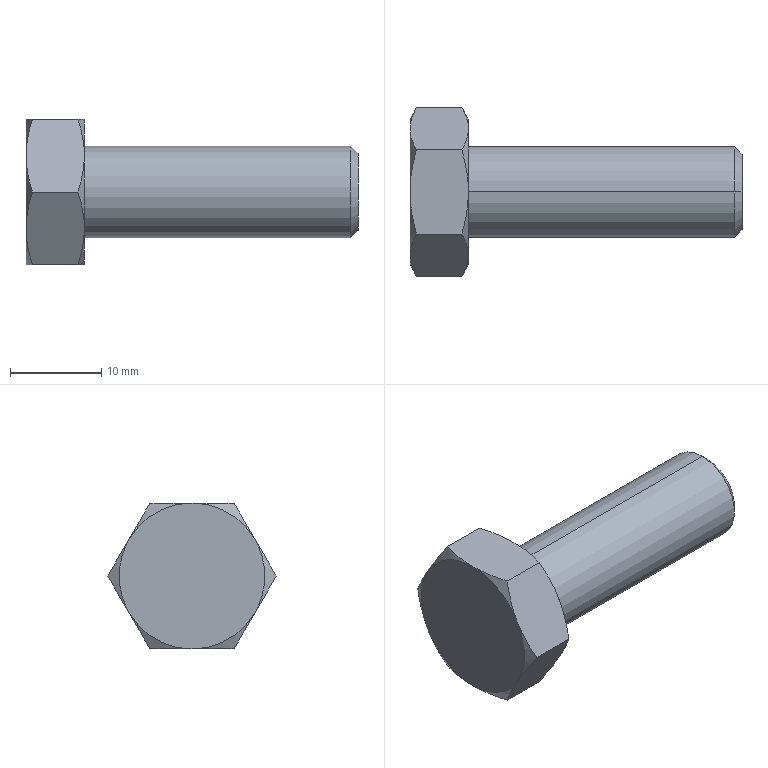Part | STEP file | Microwave Drying Flat Conveyor-screw_gb_t_6563_m10x30 | 1 solid | 25 faces | box 36.4 x 18.475 x 16 mm | volume 3756 mm3 | cone 14 | plane 9 | cylinder 2 | commonest cylinder face diameters 10 x2
STEP:
#1=CARTESIAN_POINT('',(30.,0.,4.188));
#2=VERTEX_POINT('',#1);
#3=CARTESIAN_POINT('',(30.,0.,-4.188));
#4=VERTEX_POINT('',#3);
#5=CARTESIAN_POINT('',(30.,0.,0.));
#6=DIRECTION('',(-1.,0.,0.));
#7=DIRECTION('',(0.,0.,1.));
#8=AXIS2_PLACEMENT_3D('',#5,#6,#7);
#9=CIRCLE('',#8,4.188);
#10=EDGE_CURVE('',#2,#4,#9,.T.);
#11=ORIENTED_EDGE('',*,*,#10,.T.);
#12=CARTESIAN_POINT('',(29.188,0.,-5.));
#13=VERTEX_POINT('',#12);
#14=CARTESIAN_POINT('',(29.188,0.,-5.));
#15=DIRECTION('',(-0.7071,0.,-0.7071));
#16=VECTOR('',#15,1000.);
#17=LINE('',#14,#16);
#18=EDGE_CURVE('',#4,#13,#17,.T.);
#19=ORIENTED_EDGE('',*,*,#18,.T.);
#20=CARTESIAN_POINT('',(29.188,0.,5.));
#21=VERTEX_POINT('',#20);
#22=CARTESIAN_POINT('',(29.188,0.,0.));
#23=DIRECTION('',(-1.,0.,0.));
#24=DIRECTION('',(0.,0.,1.));
#25=AXIS2_PLACEMENT_3D('',#22,#23,#24);
#26=CIRCLE('',#25,5.);
#27=EDGE_CURVE('',#21,#13,#26,.T.);
#28=ORIENTED_EDGE('',*,*,#27,.F.);
#29=CARTESIAN_POINT('',(29.188,0.,5.));
#30=DIRECTION('',(-0.7071,0.,0.7071));
#31=VECTOR('',#30,1000.);
#32=LINE('',#29,#31);
#33=EDGE_CURVE('',#2,#21,#32,.T.);
#34=ORIENTED_EDGE('',*,*,#33,.F.);
#35=EDGE_LOOP('',(#11,#19,#28,#34));
#36=FACE_OUTER_BOUND('',#35,.T.);
#37=CARTESIAN_POINT('',(29.188,0.,0.));
#38=DIRECTION('',(-1.,0.,0.));
#39=DIRECTION('',(0.,0.,1.));
#40=AXIS2_PLACEMENT_3D('',#37,#38,#39);
#41=CONICAL_SURFACE('',#40,5.,0.7854);
#42=ADVANCED_FACE('',(#36),#41,.T.);
#43=ORIENTED_EDGE('',*,*,#27,.T.);
#44=CARTESIAN_POINT('',(0.,0.,-5.));
#45=VERTEX_POINT('',#44);
#46=CARTESIAN_POINT('',(-0.1,0.,-5.));
#47=DIRECTION('',(-1.,0.,0.));
#48=VECTOR('',#47,1000.);
#49=LINE('',#46,#48);
#50=EDGE_CURVE('',#13,#45,#49,.T.);
#51=ORIENTED_EDGE('',*,*,#50,.T.);
#52=CARTESIAN_POINT('',(0.,0.,5.));
#53=VERTEX_POINT('',#52);
#54=CARTESIAN_POINT('',(0.,0.,0.));
#55=DIRECTION('',(1.,0.,0.));
#56=DIRECTION('',(0.,0.,1.));
#57=AXIS2_PLACEMENT_3D('',#54,#55,#56);
#58=CIRCLE('',#57,5.);
#59=EDGE_CURVE('',#45,#53,#58,.T.);
#60=ORIENTED_EDGE('',*,*,#59,.T.);
#61=CARTESIAN_POINT('',(-0.1,0.,5.));
#62=DIRECTION('',(-1.,0.,0.));
#63=VECTOR('',#62,1000.);
#64=LINE('',#61,#63);
#65=EDGE_CURVE('',#21,#53,#64,.T.);
#66=ORIENTED_EDGE('',*,*,#65,.F.);
#67=EDGE_LOOP('',(#43,#51,#60,#66));
#68=FACE_OUTER_BOUND('',#67,.T.);
#69=CARTESIAN_POINT('',(-0.1,0.,0.));
#70=DIRECTION('',(-1.,0.,0.));
#71=DIRECTION('',(0.,0.,1.));
#72=AXIS2_PLACEMENT_3D('',#69,#70,#71);
#73=CYLINDRICAL_SURFACE('',#72,5.);
#74=ADVANCED_FACE('',(#68),#73,.T.);
#75=ORIENTED_EDGE('',*,*,#50,.F.);
#76=CARTESIAN_POINT('',(29.188,0.,0.));
#77=DIRECTION('',(-1.,0.,0.));
#78=DIRECTION('',(0.,0.,1.));
#79=AXIS2_PLACEMENT_3D('',#76,#77,#78);
#80=CIRCLE('',#79,5.);
#81=EDGE_CURVE('',#13,#21,#80,.T.);
#82=ORIENTED_EDGE('',*,*,#81,.T.);
#83=ORIENTED_EDGE('',*,*,#65,.T.);
#84=CARTESIAN_POINT('',(0.,0.,0.));
#85=DIRECTION('',(1.,0.,0.));
#86=DIRECTION('',(0.,0.,1.));
#87=AXIS2_PLACEMENT_3D('',#84,#85,#86);
#88=CIRCLE('',#87,5.);
#89=EDGE_CURVE('',#53,#45,#88,.T.);
#90=ORIENTED_EDGE('',*,*,#89,.T.);
#91=EDGE_LOOP('',(#75,#82,#83,#90));
#92=FACE_OUTER_BOUND('',#91,.T.);
#93=CARTESIAN_POINT('',(-0.1,0.,0.));
#94=DIRECTION('',(-1.,0.,0.));
#95=DIRECTION('',(0.,0.,1.));
#96=AXIS2_PLACEMENT_3D('',#93,#94,#95);
#97=CYLINDRICAL_SURFACE('',#96,5.);
#98=ADVANCED_FACE('',(#92),#97,.T.);
#99=ORIENTED_EDGE('',*,*,#10,.F.);
#100=CARTESIAN_POINT('',(30.,0.,0.));
#101=DIRECTION('',(-1.,0.,0.));
#102=DIRECTION('',(0.,0.,1.));
#103=AXIS2_PLACEMENT_3D('',#100,#101,#102);
#104=CIRCLE('',#103,4.188);
#105=EDGE_CURVE('',#4,#2,#104,.T.);
#106=ORIENTED_EDGE('',*,*,#105,.F.);
#107=EDGE_LOOP('',(#99,#106));
#108=FACE_OUTER_BOUND('',#107,.T.);
#109=CARTESIAN_POINT('',(30.,0.,0.));
#110=DIRECTION('',(-1.,0.,0.));
#111=DIRECTION('',(0.,0.,1.));
#112=AXIS2_PLACEMENT_3D('',#109,#110,#111);
#113=PLANE('',#112);
#114=ADVANCED_FACE('',(#108),#113,.F.);
#115=ORIENTED_EDGE('',*,*,#18,.F.);
#116=ORIENTED_EDGE('',*,*,#105,.T.);
#117=ORIENTED_EDGE('',*,*,#33,.T.);
#118=ORIENTED_EDGE('',*,*,#81,.F.);
#119=EDGE_LOOP('',(#115,#116,#117,#118));
#120=FACE_OUTER_BOUND('',#119,.T.);
#121=CARTESIAN_POINT('',(29.188,0.,0.));
#122=DIRECTION('',(-1.,0.,0.));
#123=DIRECTION('',(0.,0.,1.));
#124=AXIS2_PLACEMENT_3D('',#121,#122,#123);
#125=CONICAL_SURFACE('',#124,5.,0.7854);
#126=ADVANCED_FACE('',(#120),#125,.T.);
#127=CARTESIAN_POINT('',(-0.7145,4.619,-8.));
#128=VERTEX_POINT('',#127);
#129=CARTESIAN_POINT('',(0.,0.,-8.));
#130=VERTEX_POINT('',#129);
#131=CARTESIAN_POINT('',(-0.7145,4.619,-8.));
#132=CARTESIAN_POINT('',(-0.4989,3.872,-8.));
#133=CARTESIAN_POINT('',(-0.3194,3.115,-8.));
#134=CARTESIAN_POINT('',(-0.1317,1.959,-8.));
#135=CARTESIAN_POINT('',(-0.08283,1.571,-8.));
#136=CARTESIAN_POINT('',(-0.01675,0.7849,-8.));
#137=CARTESIAN_POINT('',(0.,0.3912,-8.));
#138=CARTESIAN_POINT('',(0.,0.,-8.));
#139=B_SPLINE_CURVE_WITH_KNOTS('',3,(#131,#132,#133,#134,#135,#136,#137,#138),.UNSPECIFIED.,.F.,.F.,(4,2,2,4),(0.02228,0.02462,0.02579,0.02696),.UNSPECIFIED.);
#140=EDGE_CURVE('',#128,#130,#139,.T.);
#141=ORIENTED_EDGE('',*,*,#140,.F.);
#142=CARTESIAN_POINT('',(0.,6.928,-4.));
#143=VERTEX_POINT('',#142);
#144=CARTESIAN_POINT('',(0.,6.928,-4.));
#145=CARTESIAN_POINT('',(0.,6.732,-4.339));
#146=CARTESIAN_POINT('',(-0.01689,6.535,-4.68));
#147=CARTESIAN_POINT('',(-0.08225,6.146,-5.355));
#148=CARTESIAN_POINT('',(-0.1307,5.952,-5.69));
#149=CARTESIAN_POINT('',(-0.3174,5.376,-6.689));
#150=CARTESIAN_POINT('',(-0.497,4.996,-7.347));
#151=CARTESIAN_POINT('',(-0.7145,4.619,-8.));
#152=B_SPLINE_CURVE_WITH_KNOTS('',3,(#144,#145,#146,#147,#148,#149,#150,#151),.UNSPECIFIED.,.F.,.F.,(4,2,2,4),(0.004673,0.005837,0.007001,0.009329),.UNSPECIFIED.);
#153=EDGE_CURVE('',#143,#128,#152,.T.);
#154=ORIENTED_EDGE('',*,*,#153,.F.);
#155=CARTESIAN_POINT('',(0.,0.,0.));
#156=DIRECTION('',(-1.,0.,0.));
#157=DIRECTION('',(0.,0.,1.));
#158=AXIS2_PLACEMENT_3D('',#155,#156,#157);
#159=CIRCLE('',#158,8.);
#160=EDGE_CURVE('',#143,#130,#159,.T.);
#161=ORIENTED_EDGE('',*,*,#160,.T.);
#162=EDGE_LOOP('',(#141,#154,#161));
#163=FACE_OUTER_BOUND('',#162,.T.);
#164=CARTESIAN_POINT('',(0.,0.,0.));
#165=DIRECTION('',(-1.,0.,0.));
#166=DIRECTION('',(0.,0.,1.));
#167=AXIS2_PLACEMENT_3D('',#164,#165,#166);
#168=CONICAL_SURFACE('',#167,8.,1.047);
#169=ADVANCED_FACE('',(#163),#168,.T.);
#170=CARTESIAN_POINT('',(-0.7145,-4.619,-8.));
#171=VERTEX_POINT('',#170);
#172=CARTESIAN_POINT('',(0.,0.,-8.));
#173=CARTESIAN_POINT('',(0.,-0.7817,-8.));
#174=CARTESIAN_POINT('',(-0.06727,-1.557,-8.));
#175=CARTESIAN_POINT('',(-0.3157,-3.098,-8.));
#176=CARTESIAN_POINT('',(-0.4974,-3.866,-8.));
#177=CARTESIAN_POINT('',(-0.7145,-4.619,-8.));
#178=B_SPLINE_CURVE_WITH_KNOTS('',3,(#172,#173,#174,#175,#176,#177),.UNSPECIFIED.,.F.,.F.,(4,2,4),(0.02696,0.0293,0.03163),.UNSPECIFIED.);
#179=EDGE_CURVE('',#130,#171,#178,.T.);
#180=ORIENTED_EDGE('',*,*,#179,.F.);
#181=CARTESIAN_POINT('',(0.,-6.928,-4.));
#182=VERTEX_POINT('',#181);
#183=CARTESIAN_POINT('',(0.,0.,0.));
#184=DIRECTION('',(-1.,0.,0.));
#185=DIRECTION('',(0.,0.,1.));
#186=AXIS2_PLACEMENT_3D('',#183,#184,#185);
#187=CIRCLE('',#186,8.);
#188=EDGE_CURVE('',#130,#182,#187,.T.);
#189=ORIENTED_EDGE('',*,*,#188,.T.);
#190=CARTESIAN_POINT('',(-0.7145,-4.619,-8.));
#191=CARTESIAN_POINT('',(-0.4964,-4.997,-7.346));
#192=CARTESIAN_POINT('',(-0.3167,-5.377,-6.687));
#193=CARTESIAN_POINT('',(-0.0681,-6.146,-5.354));
#194=CARTESIAN_POINT('',(0.,-6.535,-4.681));
#195=CARTESIAN_POINT('',(0.,-6.928,-4.));
#196=B_SPLINE_CURVE_WITH_KNOTS('',3,(#190,#191,#192,#193,#194,#195),.UNSPECIFIED.,.F.,.F.,(4,2,4),(0.000000002,0.002337,0.004673),.UNSPECIFIED.);
#197=EDGE_CURVE('',#171,#182,#196,.T.);
#198=ORIENTED_EDGE('',*,*,#197,.F.);
#199=EDGE_LOOP('',(#180,#189,#198));
#200=FACE_OUTER_BOUND('',#199,.T.);
#201=CARTESIAN_POINT('',(0.,0.,0.));
#202=DIRECTION('',(-1.,0.,0.));
#203=DIRECTION('',(0.,0.,1.));
#204=AXIS2_PLACEMENT_3D('',#201,#202,#203);
#205=CONICAL_SURFACE('',#204,8.,1.047);
#206=ADVANCED_FACE('',(#200),#205,.T.);
#207=CARTESIAN_POINT('',(-0.7145,-9.238,0.));
#208=VERTEX_POINT('',#207);
#209=CARTESIAN_POINT('',(0.,-6.928,-4.));
#210=CARTESIAN_POINT('',(0.,-7.124,-3.661));
#211=CARTESIAN_POINT('',(-0.01689,-7.321,-3.32));
#212=CARTESIAN_POINT('',(-0.08225,-7.711,-2.645));
#213=CARTESIAN_POINT('',(-0.1307,-7.904,-2.31));
#214=CARTESIAN_POINT('',(-0.3174,-8.481,-1.311));
#215=CARTESIAN_POINT('',(-0.497,-8.861,-0.6527));
#216=CARTESIAN_POINT('',(-0.7145,-9.238,0.));
#217=B_SPLINE_CURVE_WITH_KNOTS('',3,(#209,#210,#211,#212,#213,#214,#215,#216),.UNSPECIFIED.,.F.,.F.,(4,2,2,4),(0.004673,0.005837,0.007001,0.009329),.UNSPECIFIED.);
#218=EDGE_CURVE('',#182,#208,#217,.T.);
#219=ORIENTED_EDGE('',*,*,#218,.F.);
#220=CARTESIAN_POINT('',(0.,-6.928,4.));
#221=VERTEX_POINT('',#220);
#222=CARTESIAN_POINT('',(0.,0.,0.));
#223=DIRECTION('',(-1.,0.,0.));
#224=DIRECTION('',(0.,0.,1.));
#225=AXIS2_PLACEMENT_3D('',#222,#223,#224);
#226=CIRCLE('',#225,8.);
#227=EDGE_CURVE('',#182,#221,#226,.T.);
#228=ORIENTED_EDGE('',*,*,#227,.T.);
#229=CARTESIAN_POINT('',(-0.7145,-9.238,0.));
#230=CARTESIAN_POINT('',(-0.4964,-8.86,0.6543));
#231=CARTESIAN_POINT('',(-0.3167,-8.479,1.313));
#232=CARTESIAN_POINT('',(-0.0681,-7.71,2.646));
#233=CARTESIAN_POINT('',(0.,-7.322,3.319));
#234=CARTESIAN_POINT('',(0.,-6.928,4.));
#235=B_SPLINE_CURVE_WITH_KNOTS('',3,(#229,#230,#231,#232,#233,#234),.UNSPECIFIED.,.F.,.F.,(4,2,4),(0.000000002,0.002337,0.004673),.UNSPECIFIED.);
#236=EDGE_CURVE('',#208,#221,#235,.T.);
#237=ORIENTED_EDGE('',*,*,#236,.F.);
#238=EDGE_LOOP('',(#219,#228,#237));
#239=FACE_OUTER_BOUND('',#238,.T.);
#240=CARTESIAN_POINT('',(0.,0.,0.));
#241=DIRECTION('',(-1.,0.,0.));
#242=DIRECTION('',(0.,0.,1.));
#243=AXIS2_PLACEMENT_3D('',#240,#241,#242);
#244=CONICAL_SURFACE('',#243,8.,1.047);
#245=ADVANCED_FACE('',(#239),#244,.T.);
#246=CARTESIAN_POINT('',(-0.7145,9.238,0.));
#247=VERTEX_POINT('',#246);
#248=CARTESIAN_POINT('',(-0.7145,9.238,0.));
#249=CARTESIAN_POINT('',(-0.4964,8.86,-0.6543));
#250=CARTESIAN_POINT('',(-0.3167,8.479,-1.313));
#251=CARTESIAN_POINT('',(-0.0681,7.71,-2.646));
#252=CARTESIAN_POINT('',(0.,7.322,-3.319));
#253=CARTESIAN_POINT('',(0.,6.928,-4.));
#254=B_SPLINE_CURVE_WITH_KNOTS('',3,(#248,#249,#250,#251,#252,#253),.UNSPECIFIED.,.F.,.F.,(4,2,4),(0.000000002,0.002337,0.004673),.UNSPECIFIED.);
#255=EDGE_CURVE('',#247,#143,#254,.T.);
#256=ORIENTED_EDGE('',*,*,#255,.F.);
#257=CARTESIAN_POINT('',(0.,6.928,4.));
#258=VERTEX_POINT('',#257);
#259=CARTESIAN_POINT('',(0.,6.928,4.));
#260=CARTESIAN_POINT('',(0.,7.124,3.661));
#261=CARTESIAN_POINT('',(-0.01689,7.321,3.32));
#262=CARTESIAN_POINT('',(-0.08225,7.711,2.645));
#263=CARTESIAN_POINT('',(-0.1307,7.904,2.31));
#264=CARTESIAN_POINT('',(-0.3174,8.481,1.311));
#265=CARTESIAN_POINT('',(-0.497,8.861,0.6527));
#266=CARTESIAN_POINT('',(-0.7145,9.238,0.));
#267=B_SPLINE_CURVE_WITH_KNOTS('',3,(#259,#260,#261,#262,#263,#264,#265,#266),.UNSPECIFIED.,.F.,.F.,(4,2,2,4),(0.004673,0.005837,0.007001,0.009329),.UNSPECIFIED.);
#268=EDGE_CURVE('',#258,#247,#267,.T.);
#269=ORIENTED_EDGE('',*,*,#268,.F.);
#270=CARTESIAN_POINT('',(0.,0.,0.));
#271=DIRECTION('',(-1.,0.,0.));
#272=DIRECTION('',(0.,0.,1.));
#273=AXIS2_PLACEMENT_3D('',#270,#271,#272);
#274=CIRCLE('',#273,8.);
#275=EDGE_CURVE('',#258,#143,#274,.T.);
#276=ORIENTED_EDGE('',*,*,#275,.T.);
#277=EDGE_LOOP('',(#256,#269,#276));
#278=FACE_OUTER_BOUND('',#277,.T.);
#279=CARTESIAN_POINT('',(0.,0.,0.));
#280=DIRECTION('',(-1.,0.,0.));
#281=DIRECTION('',(0.,0.,1.));
#282=AXIS2_PLACEMENT_3D('',#279,#280,#281);
#283=CONICAL_SURFACE('',#282,8.,1.047);
#284=ADVANCED_FACE('',(#278),#283,.T.);
#285=CARTESIAN_POINT('',(-0.7145,-4.619,8.));
#286=VERTEX_POINT('',#285);
#287=CARTESIAN_POINT('',(0.,-6.928,4.));
#288=CARTESIAN_POINT('',(0.,-6.732,4.339));
#289=CARTESIAN_POINT('',(-0.01689,-6.535,4.68));
#290=CARTESIAN_POINT('',(-0.08225,-6.146,5.355));
#291=CARTESIAN_POINT('',(-0.1307,-5.952,5.69));
#292=CARTESIAN_POINT('',(-0.3174,-5.376,6.689));
#293=CARTESIAN_POINT('',(-0.497,-4.996,7.347));
#294=CARTESIAN_POINT('',(-0.7145,-4.619,8.));
#295=B_SPLINE_CURVE_WITH_KNOTS('',3,(#287,#288,#289,#290,#291,#292,#293,#294),.UNSPECIFIED.,.F.,.F.,(4,2,2,4),(0.004673,0.005837,0.007001,0.009329),.UNSPECIFIED.);
#296=EDGE_CURVE('',#221,#286,#295,.T.);
#297=ORIENTED_EDGE('',*,*,#296,.F.);
#298=CARTESIAN_POINT('',(0.,0.,8.));
#299=VERTEX_POINT('',#298);
#300=CARTESIAN_POINT('',(0.,0.,0.));
#301=DIRECTION('',(-1.,0.,0.));
#302=DIRECTION('',(0.,0.,1.));
#303=AXIS2_PLACEMENT_3D('',#300,#301,#302);
#304=CIRCLE('',#303,8.);
#305=EDGE_CURVE('',#221,#299,#304,.T.);
#306=ORIENTED_EDGE('',*,*,#305,.T.);
#307=CARTESIAN_POINT('',(-0.7145,-4.619,8.));
#308=CARTESIAN_POINT('',(-0.4974,-3.866,8.));
#309=CARTESIAN_POINT('',(-0.3157,-3.098,8.));
#310=CARTESIAN_POINT('',(-0.06727,-1.557,8.));
#311=CARTESIAN_POINT('',(0.,-0.7817,8.));
#312=CARTESIAN_POINT('',(0.,0.,8.));
#313=B_SPLINE_CURVE_WITH_KNOTS('',3,(#307,#308,#309,#310,#311,#312),.UNSPECIFIED.,.F.,.F.,(4,2,4),(0.008627,0.01097,0.0133),.UNSPECIFIED.);
#314=EDGE_CURVE('',#286,#299,#313,.T.);
#315=ORIENTED_EDGE('',*,*,#314,.F.);
#316=EDGE_LOOP('',(#297,#306,#315));
#317=FACE_OUTER_BOUND('',#316,.T.);
#318=CARTESIAN_POINT('',(0.,0.,0.));
#319=DIRECTION('',(-1.,0.,0.));
#320=DIRECTION('',(0.,0.,1.));
#321=AXIS2_PLACEMENT_3D('',#318,#319,#320);
#322=CONICAL_SURFACE('',#321,8.,1.047);
#323=ADVANCED_FACE('',(#317),#322,.T.);
#324=CARTESIAN_POINT('',(-0.7145,4.619,8.));
#325=VERTEX_POINT('',#324);
#326=CARTESIAN_POINT('',(-0.7145,4.619,8.));
#327=CARTESIAN_POINT('',(-0.4964,4.997,7.346));
#328=CARTESIAN_POINT('',(-0.3167,5.377,6.687));
#329=CARTESIAN_POINT('',(-0.0681,6.146,5.354));
#330=CARTESIAN_POINT('',(0.,6.535,4.681));
#331=CARTESIAN_POINT('',(0.,6.928,4.));
#332=B_SPLINE_CURVE_WITH_KNOTS('',3,(#326,#327,#328,#329,#330,#331),.UNSPECIFIED.,.F.,.F.,(4,2,4),(0.000000002,0.002337,0.004673),.UNSPECIFIED.);
#333=EDGE_CURVE('',#325,#258,#332,.T.);
#334=ORIENTED_EDGE('',*,*,#333,.F.);
#335=CARTESIAN_POINT('',(0.,0.,8.));
#336=CARTESIAN_POINT('',(0.,0.3912,8.));
#337=CARTESIAN_POINT('',(-0.01675,0.7849,8.));
#338=CARTESIAN_POINT('',(-0.08283,1.571,8.));
#339=CARTESIAN_POINT('',(-0.1317,1.959,8.));
#340=CARTESIAN_POINT('',(-0.3194,3.115,8.));
#341=CARTESIAN_POINT('',(-0.4989,3.872,8.));
#342=CARTESIAN_POINT('',(-0.7145,4.619,8.));
#343=B_SPLINE_CURVE_WITH_KNOTS('',3,(#335,#336,#337,#338,#339,#340,#341,#342),.UNSPECIFIED.,.F.,.F.,(4,2,2,4),(0.0133,0.01447,0.01564,0.01798),.UNSPECIFIED.);
#344=EDGE_CURVE('',#299,#325,#343,.T.);
#345=ORIENTED_EDGE('',*,*,#344,.F.);
#346=CARTESIAN_POINT('',(0.,0.,0.));
#347=DIRECTION('',(-1.,0.,0.));
#348=DIRECTION('',(0.,0.,1.));
#349=AXIS2_PLACEMENT_3D('',#346,#347,#348);
#350=CIRCLE('',#349,8.);
#351=EDGE_CURVE('',#299,#258,#350,.T.);
#352=ORIENTED_EDGE('',*,*,#351,.T.);
#353=EDGE_LOOP('',(#334,#345,#352));
#354=FACE_OUTER_BOUND('',#353,.T.);
#355=CARTESIAN_POINT('',(0.,0.,0.));
#356=DIRECTION('',(-1.,0.,0.));
#357=DIRECTION('',(0.,0.,1.));
#358=AXIS2_PLACEMENT_3D('',#355,#356,#357);
#359=CONICAL_SURFACE('',#358,8.,1.047);
#360=ADVANCED_FACE('',(#354),#359,.T.);
#361=ORIENTED_EDGE('',*,*,#89,.F.);
#362=ORIENTED_EDGE('',*,*,#59,.F.);
#363=EDGE_LOOP('',(#361,#362));
#364=FACE_BOUND('',#363,.T.);
#365=ORIENTED_EDGE('',*,*,#351,.F.);
#366=ORIENTED_EDGE('',*,*,#305,.F.);
#367=ORIENTED_EDGE('',*,*,#227,.F.);
#368=ORIENTED_EDGE('',*,*,#188,.F.);
#369=ORIENTED_EDGE('',*,*,#160,.F.);
#370=ORIENTED_EDGE('',*,*,#275,.F.);
#371=EDGE_LOOP('',(#365,#366,#367,#368,#369,#370));
#372=FACE_OUTER_BOUND('',#371,.T.);
#373=CARTESIAN_POINT('',(0.,0.,0.));
#374=DIRECTION('',(-1.,0.,0.));
#375=DIRECTION('',(0.,0.,1.));
#376=AXIS2_PLACEMENT_3D('',#373,#374,#375);
#377=PLANE('',#376);
#378=ADVANCED_FACE('',(#364,#372),#377,.F.);
#379=CARTESIAN_POINT('',(-5.685,-9.238,0.));
#380=VERTEX_POINT('',#379);
#381=CARTESIAN_POINT('',(0.2,-9.238,0.));
#382=DIRECTION('',(-1.,0.,0.));
#383=VECTOR('',#382,1000.);
#384=LINE('',#381,#383);
#385=EDGE_CURVE('',#208,#380,#384,.T.);
#386=ORIENTED_EDGE('',*,*,#385,.F.);
#387=ORIENTED_EDGE('',*,*,#236,.T.);
#388=ORIENTED_EDGE('',*,*,#296,.T.);
#389=CARTESIAN_POINT('',(-5.685,-4.619,8.));
#390=VERTEX_POINT('',#389);
#391=CARTESIAN_POINT('',(0.2,-4.619,8.));
#392=DIRECTION('',(-1.,0.,0.));
#393=VECTOR('',#392,1000.);
#394=LINE('',#391,#393);
#395=EDGE_CURVE('',#286,#390,#394,.T.);
#396=ORIENTED_EDGE('',*,*,#395,.T.);
#397=CARTESIAN_POINT('',(-6.4,-6.928,4.));
#398=VERTEX_POINT('',#397);
#399=CARTESIAN_POINT('',(-6.4,-6.928,4.));
#400=CARTESIAN_POINT('',(-6.4,-6.732,4.339));
#401=CARTESIAN_POINT('',(-6.383,-6.535,4.68));
#402=CARTESIAN_POINT('',(-6.318,-6.146,5.355));
#403=CARTESIAN_POINT('',(-6.269,-5.952,5.69));
#404=CARTESIAN_POINT('',(-6.083,-5.376,6.689));
#405=CARTESIAN_POINT('',(-5.903,-4.996,7.347));
#406=CARTESIAN_POINT('',(-5.685,-4.619,8.));
#407=B_SPLINE_CURVE_WITH_KNOTS('',3,(#399,#400,#401,#402,#403,#404,#405,#406),.UNSPECIFIED.,.F.,.F.,(4,2,2,4),(0.004673,0.005837,0.007001,0.009329),.UNSPECIFIED.);
#408=EDGE_CURVE('',#398,#390,#407,.T.);
#409=ORIENTED_EDGE('',*,*,#408,.F.);
#410=CARTESIAN_POINT('',(-5.685,-9.238,0.));
#411=CARTESIAN_POINT('',(-5.904,-8.86,0.6543));
#412=CARTESIAN_POINT('',(-6.083,-8.479,1.313));
#413=CARTESIAN_POINT('',(-6.332,-7.71,2.646));
#414=CARTESIAN_POINT('',(-6.4,-7.322,3.319));
#415=CARTESIAN_POINT('',(-6.4,-6.928,4.));
#416=B_SPLINE_CURVE_WITH_KNOTS('',3,(#410,#411,#412,#413,#414,#415),.UNSPECIFIED.,.F.,.F.,(4,2,4),(0.000000002,0.002337,0.004673),.UNSPECIFIED.);
#417=EDGE_CURVE('',#380,#398,#416,.T.);
#418=ORIENTED_EDGE('',*,*,#417,.F.);
#419=EDGE_LOOP('',(#386,#387,#388,#396,#409,#418));
#420=FACE_OUTER_BOUND('',#419,.T.);
#421=CARTESIAN_POINT('',(0.2,-4.619,8.));
#422=DIRECTION('',(0.,0.866,-0.5));
#423=DIRECTION('',(0.,0.5,0.866));
#424=AXIS2_PLACEMENT_3D('',#421,#422,#423);
#425=PLANE('',#424);
#426=ADVANCED_FACE('',(#420),#425,.F.);
#427=CARTESIAN_POINT('',(-5.685,-4.619,-8.));
#428=VERTEX_POINT('',#427);
#429=CARTESIAN_POINT('',(0.2,-4.619,-8.));
#430=DIRECTION('',(-1.,0.,0.));
#431=VECTOR('',#430,1000.);
#432=LINE('',#429,#431);
#433=EDGE_CURVE('',#171,#428,#432,.T.);
#434=ORIENTED_EDGE('',*,*,#433,.F.);
#435=ORIENTED_EDGE('',*,*,#197,.T.);
#436=ORIENTED_EDGE('',*,*,#218,.T.);
#437=ORIENTED_EDGE('',*,*,#385,.T.);
#438=CARTESIAN_POINT('',(-6.4,-6.928,-4.));
#439=VERTEX_POINT('',#438);
#440=CARTESIAN_POINT('',(-6.4,-6.928,-4.));
#441=CARTESIAN_POINT('',(-6.4,-7.124,-3.661));
#442=CARTESIAN_POINT('',(-6.383,-7.321,-3.32));
#443=CARTESIAN_POINT('',(-6.318,-7.711,-2.645));
#444=CARTESIAN_POINT('',(-6.269,-7.904,-2.31));
#445=CARTESIAN_POINT('',(-6.083,-8.481,-1.311));
#446=CARTESIAN_POINT('',(-5.903,-8.861,-0.6527));
#447=CARTESIAN_POINT('',(-5.685,-9.238,0.));
#448=B_SPLINE_CURVE_WITH_KNOTS('',3,(#440,#441,#442,#443,#444,#445,#446,#447),.UNSPECIFIED.,.F.,.F.,(4,2,2,4),(0.004673,0.005837,0.007001,0.009329),.UNSPECIFIED.);
#449=EDGE_CURVE('',#439,#380,#448,.T.);
#450=ORIENTED_EDGE('',*,*,#449,.F.);
#451=CARTESIAN_POINT('',(-5.685,-4.619,-8.));
#452=CARTESIAN_POINT('',(-5.904,-4.997,-7.346));
#453=CARTESIAN_POINT('',(-6.083,-5.377,-6.687));
#454=CARTESIAN_POINT('',(-6.332,-6.146,-5.354));
#455=CARTESIAN_POINT('',(-6.4,-6.535,-4.681));
#456=CARTESIAN_POINT('',(-6.4,-6.928,-4.));
#457=B_SPLINE_CURVE_WITH_KNOTS('',3,(#451,#452,#453,#454,#455,#456),.UNSPECIFIED.,.F.,.F.,(4,2,4),(0.000000002,0.002337,0.004673),.UNSPECIFIED.);
#458=EDGE_CURVE('',#428,#439,#457,.T.);
#459=ORIENTED_EDGE('',*,*,#458,.F.);
#460=EDGE_LOOP('',(#434,#435,#436,#437,#450,#459));
#461=FACE_OUTER_BOUND('',#460,.T.);
#462=CARTESIAN_POINT('',(0.2,-9.238,0.));
#463=DIRECTION('',(0.,0.866,0.5));
#464=DIRECTION('',(0.,-0.5,0.866));
#465=AXIS2_PLACEMENT_3D('',#462,#463,#464);
#466=PLANE('',#465);
#467=ADVANCED_FACE('',(#461),#466,.F.);
#468=CARTESIAN_POINT('',(-5.685,4.619,-8.));
#469=VERTEX_POINT('',#468);
#470=CARTESIAN_POINT('',(0.2,4.619,-8.));
#471=DIRECTION('',(-1.,0.,0.));
#472=VECTOR('',#471,1000.);
#473=LINE('',#470,#472);
#474=EDGE_CURVE('',#128,#469,#473,.T.);
#475=ORIENTED_EDGE('',*,*,#474,.F.);
#476=ORIENTED_EDGE('',*,*,#140,.T.);
#477=ORIENTED_EDGE('',*,*,#179,.T.);
#478=ORIENTED_EDGE('',*,*,#433,.T.);
#479=CARTESIAN_POINT('',(-6.4,0.,-8.));
#480=VERTEX_POINT('',#479);
#481=CARTESIAN_POINT('',(-6.4,0.,-8.));
#482=CARTESIAN_POINT('',(-6.4,-0.7817,-8.));
#483=CARTESIAN_POINT('',(-6.333,-1.557,-8.));
#484=CARTESIAN_POINT('',(-6.084,-3.098,-8.));
#485=CARTESIAN_POINT('',(-5.903,-3.866,-8.));
#486=CARTESIAN_POINT('',(-5.685,-4.619,-8.));
#487=B_SPLINE_CURVE_WITH_KNOTS('',3,(#481,#482,#483,#484,#485,#486),.UNSPECIFIED.,.F.,.F.,(4,2,4),(0.02696,0.0293,0.03163),.UNSPECIFIED.);
#488=EDGE_CURVE('',#480,#428,#487,.T.);
#489=ORIENTED_EDGE('',*,*,#488,.F.);
#490=CARTESIAN_POINT('',(-5.685,4.619,-8.));
#491=CARTESIAN_POINT('',(-5.901,3.872,-8.));
#492=CARTESIAN_POINT('',(-6.081,3.115,-8.));
#493=CARTESIAN_POINT('',(-6.268,1.959,-8.));
#494=CARTESIAN_POINT('',(-6.317,1.571,-8.));
#495=CARTESIAN_POINT('',(-6.383,0.7849,-8.));
#496=CARTESIAN_POINT('',(-6.4,0.3912,-8.));
#497=CARTESIAN_POINT('',(-6.4,0.,-8.));
#498=B_SPLINE_CURVE_WITH_KNOTS('',3,(#490,#491,#492,#493,#494,#495,#496,#497),.UNSPECIFIED.,.F.,.F.,(4,2,2,4),(0.02228,0.02462,0.02579,0.02696),.UNSPECIFIED.);
#499=EDGE_CURVE('',#469,#480,#498,.T.);
#500=ORIENTED_EDGE('',*,*,#499,.F.);
#501=EDGE_LOOP('',(#475,#476,#477,#478,#489,#500));
#502=FACE_OUTER_BOUND('',#501,.T.);
#503=CARTESIAN_POINT('',(0.2,-4.619,-8.));
#504=DIRECTION('',(0.,0.,1.));
#505=DIRECTION('',(0.,-1.,0.));
#506=AXIS2_PLACEMENT_3D('',#503,#504,#505);
#507=PLANE('',#506);
#508=ADVANCED_FACE('',(#502),#507,.F.);
#509=CARTESIAN_POINT('',(-5.685,9.238,0.));
#510=VERTEX_POINT('',#509);
#511=CARTESIAN_POINT('',(0.2,9.238,0.));
#512=DIRECTION('',(-1.,0.,0.));
#513=VECTOR('',#512,1000.);
#514=LINE('',#511,#513);
#515=EDGE_CURVE('',#247,#510,#514,.T.);
#516=ORIENTED_EDGE('',*,*,#515,.F.);
#517=ORIENTED_EDGE('',*,*,#255,.T.);
#518=ORIENTED_EDGE('',*,*,#153,.T.);
#519=ORIENTED_EDGE('',*,*,#474,.T.);
#520=CARTESIAN_POINT('',(-6.4,6.928,-4.));
#521=VERTEX_POINT('',#520);
#522=CARTESIAN_POINT('',(-6.4,6.928,-4.));
#523=CARTESIAN_POINT('',(-6.4,6.732,-4.339));
#524=CARTESIAN_POINT('',(-6.383,6.535,-4.68));
#525=CARTESIAN_POINT('',(-6.318,6.146,-5.355));
#526=CARTESIAN_POINT('',(-6.269,5.952,-5.69));
#527=CARTESIAN_POINT('',(-6.083,5.376,-6.689));
#528=CARTESIAN_POINT('',(-5.903,4.996,-7.347));
#529=CARTESIAN_POINT('',(-5.685,4.619,-8.));
#530=B_SPLINE_CURVE_WITH_KNOTS('',3,(#522,#523,#524,#525,#526,#527,#528,#529),.UNSPECIFIED.,.F.,.F.,(4,2,2,4),(0.004673,0.005837,0.007001,0.009329),.UNSPECIFIED.);
#531=EDGE_CURVE('',#521,#469,#530,.T.);
#532=ORIENTED_EDGE('',*,*,#531,.F.);
#533=CARTESIAN_POINT('',(-5.685,9.238,0.));
#534=CARTESIAN_POINT('',(-5.904,8.86,-0.6543));
#535=CARTESIAN_POINT('',(-6.083,8.479,-1.313));
#536=CARTESIAN_POINT('',(-6.332,7.71,-2.646));
#537=CARTESIAN_POINT('',(-6.4,7.322,-3.319));
#538=CARTESIAN_POINT('',(-6.4,6.928,-4.));
#539=B_SPLINE_CURVE_WITH_KNOTS('',3,(#533,#534,#535,#536,#537,#538),.UNSPECIFIED.,.F.,.F.,(4,2,4),(0.000000002,0.002337,0.004673),.UNSPECIFIED.);
#540=EDGE_CURVE('',#510,#521,#539,.T.);
#541=ORIENTED_EDGE('',*,*,#540,.F.);
#542=EDGE_LOOP('',(#516,#517,#518,#519,#532,#541));
#543=FACE_OUTER_BOUND('',#542,.T.);
#544=CARTESIAN_POINT('',(0.2,4.619,-8.));
#545=DIRECTION('',(0.,-0.866,0.5));
#546=DIRECTION('',(0.,-0.5,-0.866));
#547=AXIS2_PLACEMENT_3D('',#544,#545,#546);
#548=PLANE('',#547);
#549=ADVANCED_FACE('',(#543),#548,.F.);
#550=CARTESIAN_POINT('',(-5.685,4.619,8.));
#551=VERTEX_POINT('',#550);
#552=CARTESIAN_POINT('',(0.2,4.619,8.));
#553=DIRECTION('',(-1.,0.,0.));
#554=VECTOR('',#553,1000.);
#555=LINE('',#552,#554);
#556=EDGE_CURVE('',#325,#551,#555,.T.);
#557=ORIENTED_EDGE('',*,*,#556,.F.);
#558=ORIENTED_EDGE('',*,*,#333,.T.);
#559=ORIENTED_EDGE('',*,*,#268,.T.);
#560=ORIENTED_EDGE('',*,*,#515,.T.);
#561=CARTESIAN_POINT('',(-6.4,6.928,4.));
#562=VERTEX_POINT('',#561);
#563=CARTESIAN_POINT('',(-6.4,6.928,4.));
#564=CARTESIAN_POINT('',(-6.4,7.124,3.661));
#565=CARTESIAN_POINT('',(-6.383,7.321,3.32));
#566=CARTESIAN_POINT('',(-6.318,7.711,2.645));
#567=CARTESIAN_POINT('',(-6.269,7.904,2.31));
#568=CARTESIAN_POINT('',(-6.083,8.481,1.311));
#569=CARTESIAN_POINT('',(-5.903,8.861,0.6527));
#570=CARTESIAN_POINT('',(-5.685,9.238,0.));
#571=B_SPLINE_CURVE_WITH_KNOTS('',3,(#563,#564,#565,#566,#567,#568,#569,#570),.UNSPECIFIED.,.F.,.F.,(4,2,2,4),(0.004673,0.005837,0.007001,0.009329),.UNSPECIFIED.);
#572=EDGE_CURVE('',#562,#510,#571,.T.);
#573=ORIENTED_EDGE('',*,*,#572,.F.);
#574=CARTESIAN_POINT('',(-5.685,4.619,8.));
#575=CARTESIAN_POINT('',(-5.904,4.997,7.346));
#576=CARTESIAN_POINT('',(-6.083,5.377,6.687));
#577=CARTESIAN_POINT('',(-6.332,6.146,5.354));
#578=CARTESIAN_POINT('',(-6.4,6.535,4.681));
#579=CARTESIAN_POINT('',(-6.4,6.928,4.));
#580=B_SPLINE_CURVE_WITH_KNOTS('',3,(#574,#575,#576,#577,#578,#579),.UNSPECIFIED.,.F.,.F.,(4,2,4),(0.000000002,0.002337,0.004673),.UNSPECIFIED.);
#581=EDGE_CURVE('',#551,#562,#580,.T.);
#582=ORIENTED_EDGE('',*,*,#581,.F.);
#583=EDGE_LOOP('',(#557,#558,#559,#560,#573,#582));
#584=FACE_OUTER_BOUND('',#583,.T.);
#585=CARTESIAN_POINT('',(0.2,9.238,0.));
#586=DIRECTION('',(0.,-0.866,-0.5));
#587=DIRECTION('',(0.,0.5,-0.866));
#588=AXIS2_PLACEMENT_3D('',#585,#586,#587);
#589=PLANE('',#588);
#590=ADVANCED_FACE('',(#584),#589,.F.);
#591=ORIENTED_EDGE('',*,*,#395,.F.);
#592=ORIENTED_EDGE('',*,*,#314,.T.);
#593=ORIENTED_EDGE('',*,*,#344,.T.);
#594=ORIENTED_EDGE('',*,*,#556,.T.);
#595=CARTESIAN_POINT('',(-6.4,0.,8.));
#596=VERTEX_POINT('',#595);
#597=CARTESIAN_POINT('',(-6.4,0.,8.));
#598=CARTESIAN_POINT('',(-6.4,0.3912,8.));
#599=CARTESIAN_POINT('',(-6.383,0.7849,8.));
#600=CARTESIAN_POINT('',(-6.317,1.571,8.));
#601=CARTESIAN_POINT('',(-6.268,1.959,8.));
#602=CARTESIAN_POINT('',(-6.081,3.115,8.));
#603=CARTESIAN_POINT('',(-5.901,3.872,8.));
#604=CARTESIAN_POINT('',(-5.685,4.619,8.));
#605=B_SPLINE_CURVE_WITH_KNOTS('',3,(#597,#598,#599,#600,#601,#602,#603,#604),.UNSPECIFIED.,.F.,.F.,(4,2,2,4),(0.0133,0.01447,0.01564,0.01798),.UNSPECIFIED.);
#606=EDGE_CURVE('',#596,#551,#605,.T.);
#607=ORIENTED_EDGE('',*,*,#606,.F.);
#608=CARTESIAN_POINT('',(-5.685,-4.619,8.));
#609=CARTESIAN_POINT('',(-5.903,-3.866,8.));
#610=CARTESIAN_POINT('',(-6.084,-3.098,8.));
#611=CARTESIAN_POINT('',(-6.333,-1.557,8.));
#612=CARTESIAN_POINT('',(-6.4,-0.7817,8.));
#613=CARTESIAN_POINT('',(-6.4,0.,8.));
#614=B_SPLINE_CURVE_WITH_KNOTS('',3,(#608,#609,#610,#611,#612,#613),.UNSPECIFIED.,.F.,.F.,(4,2,4),(0.008627,0.01097,0.0133),.UNSPECIFIED.);
#615=EDGE_CURVE('',#390,#596,#614,.T.);
#616=ORIENTED_EDGE('',*,*,#615,.F.);
#617=EDGE_LOOP('',(#591,#592,#593,#594,#607,#616));
#618=FACE_OUTER_BOUND('',#617,.T.);
#619=CARTESIAN_POINT('',(0.2,4.619,8.));
#620=DIRECTION('',(0.,0.,-1.));
#621=DIRECTION('',(0.,1.,0.));
#622=AXIS2_PLACEMENT_3D('',#619,#620,#621);
#623=PLANE('',#622);
#624=ADVANCED_FACE('',(#618),#623,.F.);
#625=CARTESIAN_POINT('',(-6.4,0.,0.));
#626=DIRECTION('',(-1.,0.,0.));
#627=DIRECTION('',(0.,0.,1.));
#628=AXIS2_PLACEMENT_3D('',#625,#626,#627);
#629=CIRCLE('',#628,8.);
#630=EDGE_CURVE('',#398,#596,#629,.T.);
#631=ORIENTED_EDGE('',*,*,#630,.F.);
#632=ORIENTED_EDGE('',*,*,#408,.T.);
#633=ORIENTED_EDGE('',*,*,#615,.T.);
#634=EDGE_LOOP('',(#631,#632,#633));
#635=FACE_OUTER_BOUND('',#634,.T.);
#636=CARTESIAN_POINT('',(-6.4,0.,0.));
#637=DIRECTION('',(1.,0.,0.));
#638=DIRECTION('',(0.,0.,-1.));
#639=AXIS2_PLACEMENT_3D('',#636,#637,#638);
#640=CONICAL_SURFACE('',#639,8.,1.047);
#641=ADVANCED_FACE('',(#635),#640,.T.);
#642=CARTESIAN_POINT('',(-6.4,0.,0.));
#643=DIRECTION('',(-1.,0.,0.));
#644=DIRECTION('',(0.,0.,1.));
#645=AXIS2_PLACEMENT_3D('',#642,#643,#644);
#646=CIRCLE('',#645,8.);
#647=EDGE_CURVE('',#439,#398,#646,.T.);
#648=ORIENTED_EDGE('',*,*,#647,.F.);
#649=ORIENTED_EDGE('',*,*,#449,.T.);
#650=ORIENTED_EDGE('',*,*,#417,.T.);
#651=EDGE_LOOP('',(#648,#649,#650));
#652=FACE_OUTER_BOUND('',#651,.T.);
#653=CARTESIAN_POINT('',(-6.4,0.,0.));
#654=DIRECTION('',(1.,0.,0.));
#655=DIRECTION('',(0.,0.,-1.));
#656=AXIS2_PLACEMENT_3D('',#653,#654,#655);
#657=CONICAL_SURFACE('',#656,8.,1.047);
#658=ADVANCED_FACE('',(#652),#657,.T.);
#659=CARTESIAN_POINT('',(-6.4,0.,0.));
#660=DIRECTION('',(-1.,0.,0.));
#661=DIRECTION('',(0.,0.,1.));
#662=AXIS2_PLACEMENT_3D('',#659,#660,#661);
#663=CIRCLE('',#662,8.);
#664=EDGE_CURVE('',#480,#439,#663,.T.);
#665=ORIENTED_EDGE('',*,*,#664,.F.);
#666=ORIENTED_EDGE('',*,*,#488,.T.);
#667=ORIENTED_EDGE('',*,*,#458,.T.);
#668=EDGE_LOOP('',(#665,#666,#667));
#669=FACE_OUTER_BOUND('',#668,.T.);
#670=CARTESIAN_POINT('',(-6.4,0.,0.));
#671=DIRECTION('',(1.,0.,0.));
#672=DIRECTION('',(0.,0.,-1.));
#673=AXIS2_PLACEMENT_3D('',#670,#671,#672);
#674=CONICAL_SURFACE('',#673,8.,1.047);
#675=ADVANCED_FACE('',(#669),#674,.T.);
#676=ORIENTED_EDGE('',*,*,#531,.T.);
#677=ORIENTED_EDGE('',*,*,#499,.T.);
#678=CARTESIAN_POINT('',(-6.4,0.,0.));
#679=DIRECTION('',(-1.,0.,0.));
#680=DIRECTION('',(0.,0.,1.));
#681=AXIS2_PLACEMENT_3D('',#678,#679,#680);
#682=CIRCLE('',#681,8.);
#683=EDGE_CURVE('',#521,#480,#682,.T.);
#684=ORIENTED_EDGE('',*,*,#683,.F.);
#685=EDGE_LOOP('',(#676,#677,#684));
#686=FACE_OUTER_BOUND('',#685,.T.);
#687=CARTESIAN_POINT('',(-6.4,0.,0.));
#688=DIRECTION('',(1.,0.,0.));
#689=DIRECTION('',(0.,0.,-1.));
#690=AXIS2_PLACEMENT_3D('',#687,#688,#689);
#691=CONICAL_SURFACE('',#690,8.,1.047);
#692=ADVANCED_FACE('',(#686),#691,.T.);
#693=ORIENTED_EDGE('',*,*,#572,.T.);
#694=ORIENTED_EDGE('',*,*,#540,.T.);
#695=CARTESIAN_POINT('',(-6.4,0.,0.));
#696=DIRECTION('',(-1.,0.,0.));
#697=DIRECTION('',(0.,0.,1.));
#698=AXIS2_PLACEMENT_3D('',#695,#696,#697);
#699=CIRCLE('',#698,8.);
#700=EDGE_CURVE('',#562,#521,#699,.T.);
#701=ORIENTED_EDGE('',*,*,#700,.F.);
#702=EDGE_LOOP('',(#693,#694,#701));
#703=FACE_OUTER_BOUND('',#702,.T.);
#704=CARTESIAN_POINT('',(-6.4,0.,0.));
#705=DIRECTION('',(1.,0.,0.));
#706=DIRECTION('',(0.,0.,-1.));
#707=AXIS2_PLACEMENT_3D('',#704,#705,#706);
#708=CONICAL_SURFACE('',#707,8.,1.047);
#709=ADVANCED_FACE('',(#703),#708,.T.);
#710=CARTESIAN_POINT('',(-6.4,0.,0.));
#711=DIRECTION('',(-1.,0.,0.));
#712=DIRECTION('',(0.,0.,1.));
#713=AXIS2_PLACEMENT_3D('',#710,#711,#712);
#714=CIRCLE('',#713,8.);
#715=EDGE_CURVE('',#596,#562,#714,.T.);
#716=ORIENTED_EDGE('',*,*,#715,.T.);
#717=ORIENTED_EDGE('',*,*,#700,.T.);
#718=ORIENTED_EDGE('',*,*,#683,.T.);
#719=ORIENTED_EDGE('',*,*,#664,.T.);
#720=ORIENTED_EDGE('',*,*,#647,.T.);
#721=ORIENTED_EDGE('',*,*,#630,.T.);
#722=EDGE_LOOP('',(#716,#717,#718,#719,#720,#721));
#723=FACE_OUTER_BOUND('',#722,.T.);
#724=CARTESIAN_POINT('',(-6.4,0.,0.));
#725=DIRECTION('',(-1.,0.,0.));
#726=DIRECTION('',(0.,0.,1.));
#727=AXIS2_PLACEMENT_3D('',#724,#725,#726);
#728=PLANE('',#727);
#729=ADVANCED_FACE('',(#723),#728,.T.);
#730=ORIENTED_EDGE('',*,*,#606,.T.);
#731=ORIENTED_EDGE('',*,*,#581,.T.);
#732=ORIENTED_EDGE('',*,*,#715,.F.);
#733=EDGE_LOOP('',(#730,#731,#732));
#734=FACE_OUTER_BOUND('',#733,.T.);
#735=CARTESIAN_POINT('',(-6.4,0.,0.));
#736=DIRECTION('',(1.,0.,0.));
#737=DIRECTION('',(0.,0.,-1.));
#738=AXIS2_PLACEMENT_3D('',#735,#736,#737);
#739=CONICAL_SURFACE('',#738,8.,1.047);
#740=ADVANCED_FACE('',(#734),#739,.T.);
#741=CLOSED_SHELL('',(#42,#74,#98,#114,#126,#169,#206,#245,#284,#323,#360,#378,#426,#467,#508,#549,#590,#624,#641,#658,#675,#692,#709,#729,#740));
#742=MANIFOLD_SOLID_BREP('',#741);
#743=CARTESIAN_POINT('',(0.,0.,0.));
#744=DIRECTION('',(0.,0.,1.));
#745=DIRECTION('',(1.,0.,0.));
#746=AXIS2_PLACEMENT_3D('',#743,#744,#745);
#747=(LENGTH_UNIT()NAMED_UNIT(*)SI_UNIT(.MILLI.,.METRE.));
#748=UNCERTAINTY_MEASURE_WITH_UNIT(LENGTH_MEASURE(0.00001),#747,'','');
#749=(NAMED_UNIT(*)PLANE_ANGLE_UNIT()SI_UNIT($,.RADIAN.));
#750=(NAMED_UNIT(*)SI_UNIT($,.STERADIAN.)SOLID_ANGLE_UNIT());
#751=(GEOMETRIC_REPRESENTATION_CONTEXT(3)GLOBAL_UNCERTAINTY_ASSIGNED_CONTEXT((#748))GLOBAL_UNIT_ASSIGNED_CONTEXT((#747,#749,#750))REPRESENTATION_CONTEXT('',''));
#752=ADVANCED_BREP_SHAPE_REPRESENTATION('',(#742,#746),#751);